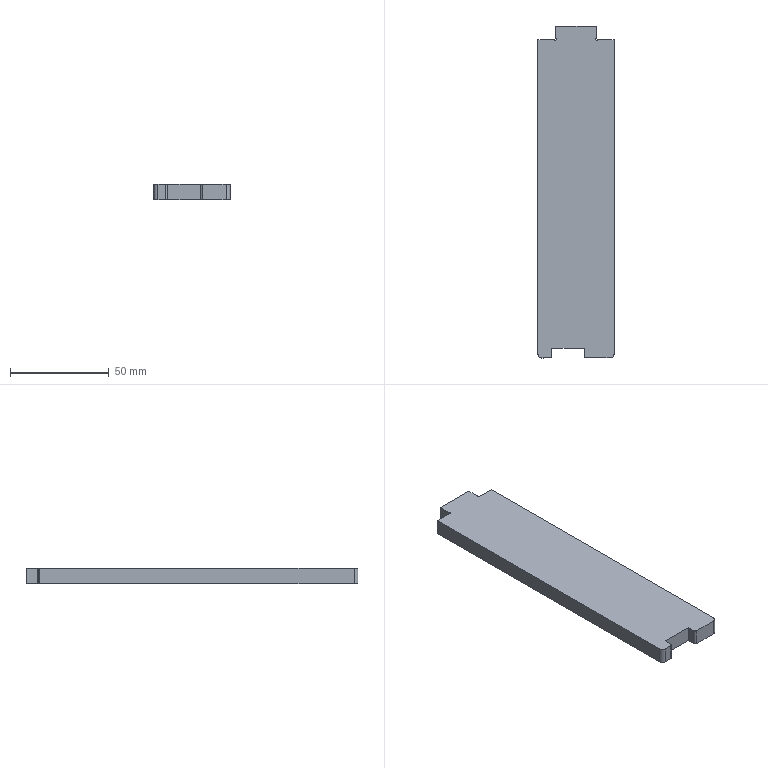Part | SolidWorks | features Fillet 2, FlatPattern 1, ICE 1, SMBaseFlange 1, SheetMetal 1 | 1 solid | 25 faces | box 38.5 x 167.8 x 8 mm | volume 49992 mm3 | plane 14 | cylinder 11 | commonest cylinder face diameters 2 x6 1 x3 4 x2
STEP:
#1=CARTESIAN_POINT('',(-109.914,161.326,-8.));
#2=VERTEX_POINT('',#1);
#3=CARTESIAN_POINT('',(-109.831,161.05,-8.));
#4=VERTEX_POINT('',#3);
#5=CARTESIAN_POINT('',(-110.331,161.05,-8.));
#6=DIRECTION('',(0.,0.,-1.));
#7=DIRECTION('',(-1.,0.,0.));
#8=AXIS2_PLACEMENT_3D('',#5,#6,#7);
#9=CIRCLE('',#8,0.5);
#10=EDGE_CURVE('',#2,#4,#9,.T.);
#11=ORIENTED_EDGE('',*,*,#10,.T.);
#12=CARTESIAN_POINT('',(-109.831,161.05,0.));
#13=VERTEX_POINT('',#12);
#14=CARTESIAN_POINT('',(-109.831,161.05,-8.));
#15=DIRECTION('',(0.,0.,1.));
#16=VECTOR('',#15,1000.);
#17=LINE('',#14,#16);
#18=EDGE_CURVE('',#4,#13,#17,.T.);
#19=ORIENTED_EDGE('',*,*,#18,.T.);
#20=CARTESIAN_POINT('',(-109.914,161.326,0.));
#21=VERTEX_POINT('',#20);
#22=CARTESIAN_POINT('',(-110.331,161.05,0.));
#23=DIRECTION('',(0.,0.,-1.));
#24=DIRECTION('',(-1.,0.,0.));
#25=AXIS2_PLACEMENT_3D('',#22,#23,#24);
#26=CIRCLE('',#25,0.5);
#27=EDGE_CURVE('',#21,#13,#26,.T.);
#28=ORIENTED_EDGE('',*,*,#27,.F.);
#29=CARTESIAN_POINT('',(-109.914,161.326,-8.));
#30=DIRECTION('',(0.,0.,-1.));
#31=VECTOR('',#30,1000.);
#32=LINE('',#29,#31);
#33=EDGE_CURVE('',#21,#2,#32,.T.);
#34=ORIENTED_EDGE('',*,*,#33,.T.);
#35=EDGE_LOOP('',(#11,#19,#28,#34));
#36=FACE_OUTER_BOUND('',#35,.T.);
#37=CARTESIAN_POINT('',(-110.331,161.05,-8.));
#38=DIRECTION('',(0.,0.,1.));
#39=DIRECTION('',(1.,0.,0.));
#40=AXIS2_PLACEMENT_3D('',#37,#38,#39);
#41=CYLINDRICAL_SURFACE('',#40,0.5);
#42=ADVANCED_FACE('',(#36),#41,.F.);
#43=CARTESIAN_POINT('',(-111.16,160.8,0.));
#44=VERTEX_POINT('',#43);
#45=CARTESIAN_POINT('',(-119.081,160.8,0.));
#46=VERTEX_POINT('',#45);
#47=CARTESIAN_POINT('',(-110.081,160.8,0.));
#48=DIRECTION('',(-1.,0.,0.));
#49=VECTOR('',#48,1000.);
#50=LINE('',#47,#49);
#51=EDGE_CURVE('',#44,#46,#50,.T.);
#52=ORIENTED_EDGE('',*,*,#51,.F.);
#53=CARTESIAN_POINT('',(-111.16,160.8,-8.));
#54=VERTEX_POINT('',#53);
#55=CARTESIAN_POINT('',(-111.16,160.8,-8.));
#56=DIRECTION('',(0.,0.,-1.));
#57=VECTOR('',#56,1000.);
#58=LINE('',#55,#57);
#59=EDGE_CURVE('',#44,#54,#58,.T.);
#60=ORIENTED_EDGE('',*,*,#59,.T.);
#61=CARTESIAN_POINT('',(-119.081,160.8,-8.));
#62=VERTEX_POINT('',#61);
#63=CARTESIAN_POINT('',(-110.081,160.8,-8.));
#64=DIRECTION('',(-1.,0.,0.));
#65=VECTOR('',#64,1000.);
#66=LINE('',#63,#65);
#67=EDGE_CURVE('',#54,#62,#66,.T.);
#68=ORIENTED_EDGE('',*,*,#67,.T.);
#69=CARTESIAN_POINT('',(-119.081,160.8,-8.));
#70=DIRECTION('',(0.,0.,1.));
#71=VECTOR('',#70,1000.);
#72=LINE('',#69,#71);
#73=EDGE_CURVE('',#62,#46,#72,.T.);
#74=ORIENTED_EDGE('',*,*,#73,.T.);
#75=EDGE_LOOP('',(#52,#60,#68,#74));
#76=FACE_OUTER_BOUND('',#75,.T.);
#77=CARTESIAN_POINT('',(-110.081,160.8,-8.));
#78=DIRECTION('',(0.,1.,0.));
#79=DIRECTION('',(0.,0.,1.));
#80=AXIS2_PLACEMENT_3D('',#77,#78,#79);
#81=PLANE('',#80);
#82=ADVANCED_FACE('',(#76),#81,.T.);
#83=CARTESIAN_POINT('',(-110.081,167.8,-8.));
#84=VERTEX_POINT('',#83);
#85=CARTESIAN_POINT('',(-110.081,161.879,-8.));
#86=VERTEX_POINT('',#85);
#87=CARTESIAN_POINT('',(-110.081,160.8,-8.));
#88=DIRECTION('',(0.,-1.,0.));
#89=VECTOR('',#88,1000.);
#90=LINE('',#87,#89);
#91=EDGE_CURVE('',#84,#86,#90,.T.);
#92=ORIENTED_EDGE('',*,*,#91,.T.);
#93=CARTESIAN_POINT('',(-110.081,161.879,0.));
#94=VERTEX_POINT('',#93);
#95=CARTESIAN_POINT('',(-110.081,161.879,-8.));
#96=DIRECTION('',(0.,0.,1.));
#97=VECTOR('',#96,1000.);
#98=LINE('',#95,#97);
#99=EDGE_CURVE('',#86,#94,#98,.T.);
#100=ORIENTED_EDGE('',*,*,#99,.T.);
#101=CARTESIAN_POINT('',(-110.081,167.8,0.));
#102=VERTEX_POINT('',#101);
#103=CARTESIAN_POINT('',(-110.081,160.8,0.));
#104=DIRECTION('',(0.,-1.,0.));
#105=VECTOR('',#104,1000.);
#106=LINE('',#103,#105);
#107=EDGE_CURVE('',#102,#94,#106,.T.);
#108=ORIENTED_EDGE('',*,*,#107,.F.);
#109=CARTESIAN_POINT('',(-110.081,167.8,-8.));
#110=DIRECTION('',(0.,0.,1.));
#111=VECTOR('',#110,1000.);
#112=LINE('',#109,#111);
#113=EDGE_CURVE('',#84,#102,#112,.T.);
#114=ORIENTED_EDGE('',*,*,#113,.F.);
#115=EDGE_LOOP('',(#92,#100,#108,#114));
#116=FACE_OUTER_BOUND('',#115,.T.);
#117=CARTESIAN_POINT('',(-110.081,160.8,-8.));
#118=DIRECTION('',(-1.,0.,0.));
#119=DIRECTION('',(0.,0.,1.));
#120=AXIS2_PLACEMENT_3D('',#117,#118,#119);
#121=PLANE('',#120);
#122=ADVANCED_FACE('',(#116),#121,.T.);
#123=CARTESIAN_POINT('',(-89.581,161.879,0.));
#124=VERTEX_POINT('',#123);
#125=CARTESIAN_POINT('',(-89.581,167.8,0.));
#126=VERTEX_POINT('',#125);
#127=CARTESIAN_POINT('',(-89.581,167.8,0.));
#128=DIRECTION('',(0.,1.,0.));
#129=VECTOR('',#128,1000.);
#130=LINE('',#127,#129);
#131=EDGE_CURVE('',#124,#126,#130,.T.);
#132=ORIENTED_EDGE('',*,*,#131,.F.);
#133=CARTESIAN_POINT('',(-89.581,161.879,-8.));
#134=VERTEX_POINT('',#133);
#135=CARTESIAN_POINT('',(-89.581,161.879,-8.));
#136=DIRECTION('',(0.,0.,-1.));
#137=VECTOR('',#136,1000.);
#138=LINE('',#135,#137);
#139=EDGE_CURVE('',#124,#134,#138,.T.);
#140=ORIENTED_EDGE('',*,*,#139,.T.);
#141=CARTESIAN_POINT('',(-89.581,167.8,-8.));
#142=VERTEX_POINT('',#141);
#143=CARTESIAN_POINT('',(-89.581,167.8,-8.));
#144=DIRECTION('',(0.,1.,0.));
#145=VECTOR('',#144,1000.);
#146=LINE('',#143,#145);
#147=EDGE_CURVE('',#134,#142,#146,.T.);
#148=ORIENTED_EDGE('',*,*,#147,.T.);
#149=CARTESIAN_POINT('',(-89.581,167.8,-8.));
#150=DIRECTION('',(0.,0.,1.));
#151=VECTOR('',#150,1000.);
#152=LINE('',#149,#151);
#153=EDGE_CURVE('',#142,#126,#152,.T.);
#154=ORIENTED_EDGE('',*,*,#153,.T.);
#155=EDGE_LOOP('',(#132,#140,#148,#154));
#156=FACE_OUTER_BOUND('',#155,.T.);
#157=CARTESIAN_POINT('',(-89.581,167.8,-8.));
#158=DIRECTION('',(1.,0.,0.));
#159=DIRECTION('',(0.,0.,-1.));
#160=AXIS2_PLACEMENT_3D('',#157,#158,#159);
#161=PLANE('',#160);
#162=ADVANCED_FACE('',(#156),#161,.T.);
#163=CARTESIAN_POINT('',(-80.581,160.8,-8.));
#164=VERTEX_POINT('',#163);
#165=CARTESIAN_POINT('',(-88.502,160.8,-8.));
#166=VERTEX_POINT('',#165);
#167=CARTESIAN_POINT('',(-80.581,160.8,-8.));
#168=DIRECTION('',(-1.,0.,0.));
#169=VECTOR('',#168,1000.);
#170=LINE('',#167,#169);
#171=EDGE_CURVE('',#164,#166,#170,.T.);
#172=ORIENTED_EDGE('',*,*,#171,.T.);
#173=CARTESIAN_POINT('',(-88.502,160.8,0.));
#174=VERTEX_POINT('',#173);
#175=CARTESIAN_POINT('',(-88.502,160.8,-8.));
#176=DIRECTION('',(0.,0.,1.));
#177=VECTOR('',#176,1000.);
#178=LINE('',#175,#177);
#179=EDGE_CURVE('',#166,#174,#178,.T.);
#180=ORIENTED_EDGE('',*,*,#179,.T.);
#181=CARTESIAN_POINT('',(-80.581,160.8,0.));
#182=VERTEX_POINT('',#181);
#183=CARTESIAN_POINT('',(-80.581,160.8,0.));
#184=DIRECTION('',(-1.,0.,0.));
#185=VECTOR('',#184,1000.);
#186=LINE('',#183,#185);
#187=EDGE_CURVE('',#182,#174,#186,.T.);
#188=ORIENTED_EDGE('',*,*,#187,.F.);
#189=CARTESIAN_POINT('',(-80.581,160.8,-8.));
#190=DIRECTION('',(0.,0.,1.));
#191=VECTOR('',#190,1000.);
#192=LINE('',#189,#191);
#193=EDGE_CURVE('',#164,#182,#192,.T.);
#194=ORIENTED_EDGE('',*,*,#193,.F.);
#195=EDGE_LOOP('',(#172,#180,#188,#194));
#196=FACE_OUTER_BOUND('',#195,.T.);
#197=CARTESIAN_POINT('',(-80.581,160.8,-8.));
#198=DIRECTION('',(0.,1.,0.));
#199=DIRECTION('',(0.,0.,1.));
#200=AXIS2_PLACEMENT_3D('',#197,#198,#199);
#201=PLANE('',#200);
#202=ADVANCED_FACE('',(#196),#201,.T.);
#203=CARTESIAN_POINT('',(-80.581,2.,-8.));
#204=VERTEX_POINT('',#203);
#205=CARTESIAN_POINT('',(-80.581,0.,-8.));
#206=DIRECTION('',(0.,1.,0.));
#207=VECTOR('',#206,1000.);
#208=LINE('',#205,#207);
#209=EDGE_CURVE('',#204,#164,#208,.T.);
#210=ORIENTED_EDGE('',*,*,#209,.F.);
#211=CARTESIAN_POINT('',(-82.581,0.,-8.));
#212=VERTEX_POINT('',#211);
#213=CARTESIAN_POINT('',(-82.581,2.,-8.));
#214=DIRECTION('',(0.,0.,-1.));
#215=DIRECTION('',(1.,0.,0.));
#216=AXIS2_PLACEMENT_3D('',#213,#214,#215);
#217=CIRCLE('',#216,2.);
#218=EDGE_CURVE('',#204,#212,#217,.T.);
#219=ORIENTED_EDGE('',*,*,#218,.T.);
#220=CARTESIAN_POINT('',(-94.581,0.,-8.));
#221=VERTEX_POINT('',#220);
#222=CARTESIAN_POINT('',(-95.581,0.,-8.));
#223=DIRECTION('',(1.,0.,0.));
#224=VECTOR('',#223,1000.);
#225=LINE('',#222,#224);
#226=EDGE_CURVE('',#221,#212,#225,.T.);
#227=ORIENTED_EDGE('',*,*,#226,.F.);
#228=CARTESIAN_POINT('',(-95.581,1.,-8.));
#229=VERTEX_POINT('',#228);
#230=CARTESIAN_POINT('',(-94.581,1.,-8.));
#231=DIRECTION('',(0.,0.,-1.));
#232=DIRECTION('',(1.,0.,0.));
#233=AXIS2_PLACEMENT_3D('',#230,#231,#232);
#234=CIRCLE('',#233,1.);
#235=EDGE_CURVE('',#221,#229,#234,.T.);
#236=ORIENTED_EDGE('',*,*,#235,.T.);
#237=CARTESIAN_POINT('',(-95.581,5.,-8.));
#238=VERTEX_POINT('',#237);
#239=CARTESIAN_POINT('',(-95.581,5.,-8.));
#240=DIRECTION('',(0.,-1.,0.));
#241=VECTOR('',#240,1000.);
#242=LINE('',#239,#241);
#243=EDGE_CURVE('',#238,#229,#242,.T.);
#244=ORIENTED_EDGE('',*,*,#243,.F.);
#245=CARTESIAN_POINT('',(-112.081,5.,-8.));
#246=VERTEX_POINT('',#245);
#247=CARTESIAN_POINT('',(-95.581,5.,-8.));
#248=DIRECTION('',(1.,0.,0.));
#249=VECTOR('',#248,1000.);
#250=LINE('',#247,#249);
#251=EDGE_CURVE('',#246,#238,#250,.T.);
#252=ORIENTED_EDGE('',*,*,#251,.F.);
#253=CARTESIAN_POINT('',(-112.081,1.,-8.));
#254=VERTEX_POINT('',#253);
#255=CARTESIAN_POINT('',(-112.081,5.,-8.));
#256=DIRECTION('',(0.,1.,0.));
#257=VECTOR('',#256,1000.);
#258=LINE('',#255,#257);
#259=EDGE_CURVE('',#254,#246,#258,.T.);
#260=ORIENTED_EDGE('',*,*,#259,.F.);
#261=CARTESIAN_POINT('',(-113.081,0.,-8.));
#262=VERTEX_POINT('',#261);
#263=CARTESIAN_POINT('',(-113.081,1.,-8.));
#264=DIRECTION('',(0.,0.,-1.));
#265=DIRECTION('',(1.,0.,0.));
#266=AXIS2_PLACEMENT_3D('',#263,#264,#265);
#267=CIRCLE('',#266,1.);
#268=EDGE_CURVE('',#254,#262,#267,.T.);
#269=ORIENTED_EDGE('',*,*,#268,.T.);
#270=CARTESIAN_POINT('',(-117.081,0.,-8.));
#271=VERTEX_POINT('',#270);
#272=CARTESIAN_POINT('',(-112.081,0.,-8.));
#273=DIRECTION('',(1.,0.,0.));
#274=VECTOR('',#273,1000.);
#275=LINE('',#272,#274);
#276=EDGE_CURVE('',#271,#262,#275,.T.);
#277=ORIENTED_EDGE('',*,*,#276,.F.);
#278=CARTESIAN_POINT('',(-119.081,2.,-8.));
#279=VERTEX_POINT('',#278);
#280=CARTESIAN_POINT('',(-117.081,2.,-8.));
#281=DIRECTION('',(0.,0.,-1.));
#282=DIRECTION('',(1.,0.,0.));
#283=AXIS2_PLACEMENT_3D('',#280,#281,#282);
#284=CIRCLE('',#283,2.);
#285=EDGE_CURVE('',#271,#279,#284,.T.);
#286=ORIENTED_EDGE('',*,*,#285,.T.);
#287=CARTESIAN_POINT('',(-119.081,0.,-8.));
#288=DIRECTION('',(0.,-1.,0.));
#289=VECTOR('',#288,1000.);
#290=LINE('',#287,#289);
#291=EDGE_CURVE('',#62,#279,#290,.T.);
#292=ORIENTED_EDGE('',*,*,#291,.F.);
#293=ORIENTED_EDGE('',*,*,#67,.F.);
#294=CARTESIAN_POINT('',(-110.607,160.633,-8.));
#295=VERTEX_POINT('',#294);
#296=CARTESIAN_POINT('',(-111.16,159.8,-8.));
#297=DIRECTION('',(0.,0.,-1.));
#298=DIRECTION('',(1.,0.,0.));
#299=AXIS2_PLACEMENT_3D('',#296,#297,#298);
#300=CIRCLE('',#299,1.);
#301=EDGE_CURVE('',#54,#295,#300,.T.);
#302=ORIENTED_EDGE('',*,*,#301,.T.);
#303=CARTESIAN_POINT('',(-110.331,161.05,-8.));
#304=DIRECTION('',(0.,0.,-1.));
#305=DIRECTION('',(-1.,0.,0.));
#306=AXIS2_PLACEMENT_3D('',#303,#304,#305);
#307=CIRCLE('',#306,0.5);
#308=EDGE_CURVE('',#4,#295,#307,.T.);
#309=ORIENTED_EDGE('',*,*,#308,.F.);
#310=ORIENTED_EDGE('',*,*,#10,.F.);
#311=CARTESIAN_POINT('',(-109.081,161.879,-8.));
#312=DIRECTION('',(0.,0.,-1.));
#313=DIRECTION('',(1.,0.,0.));
#314=AXIS2_PLACEMENT_3D('',#311,#312,#313);
#315=CIRCLE('',#314,1.);
#316=EDGE_CURVE('',#2,#86,#315,.T.);
#317=ORIENTED_EDGE('',*,*,#316,.T.);
#318=ORIENTED_EDGE('',*,*,#91,.F.);
#319=CARTESIAN_POINT('',(-110.081,167.8,-8.));
#320=DIRECTION('',(-1.,0.,0.));
#321=VECTOR('',#320,1000.);
#322=LINE('',#319,#321);
#323=EDGE_CURVE('',#142,#84,#322,.T.);
#324=ORIENTED_EDGE('',*,*,#323,.F.);
#325=ORIENTED_EDGE('',*,*,#147,.F.);
#326=CARTESIAN_POINT('',(-89.747,161.326,-8.));
#327=VERTEX_POINT('',#326);
#328=CARTESIAN_POINT('',(-90.581,161.879,-8.));
#329=DIRECTION('',(0.,0.,-1.));
#330=DIRECTION('',(1.,0.,0.));
#331=AXIS2_PLACEMENT_3D('',#328,#329,#330);
#332=CIRCLE('',#331,1.);
#333=EDGE_CURVE('',#134,#327,#332,.T.);
#334=ORIENTED_EDGE('',*,*,#333,.T.);
#335=CARTESIAN_POINT('',(-89.054,160.633,-8.));
#336=VERTEX_POINT('',#335);
#337=CARTESIAN_POINT('',(-89.331,161.05,-8.));
#338=DIRECTION('',(0.,0.,-1.));
#339=DIRECTION('',(-1.,0.,0.));
#340=AXIS2_PLACEMENT_3D('',#337,#338,#339);
#341=CIRCLE('',#340,0.5);
#342=EDGE_CURVE('',#336,#327,#341,.T.);
#343=ORIENTED_EDGE('',*,*,#342,.F.);
#344=CARTESIAN_POINT('',(-88.502,159.8,-8.));
#345=DIRECTION('',(0.,0.,-1.));
#346=DIRECTION('',(1.,0.,0.));
#347=AXIS2_PLACEMENT_3D('',#344,#345,#346);
#348=CIRCLE('',#347,1.);
#349=EDGE_CURVE('',#336,#166,#348,.T.);
#350=ORIENTED_EDGE('',*,*,#349,.T.);
#351=ORIENTED_EDGE('',*,*,#171,.F.);
#352=EDGE_LOOP('',(#210,#219,#227,#236,#244,#252,#260,#269,#277,#286,#292,#293,#302,#309,#310,#317,#318,#324,#325,#334,#343,#350,#351));
#353=FACE_OUTER_BOUND('',#352,.T.);
#354=CARTESIAN_POINT('',(0.,0.,-8.));
#355=DIRECTION('',(0.,0.,1.));
#356=DIRECTION('',(1.,0.,0.));
#357=AXIS2_PLACEMENT_3D('',#354,#355,#356);
#358=PLANE('',#357);
#359=ADVANCED_FACE('',(#353),#358,.F.);
#360=CARTESIAN_POINT('',(-94.581,0.,0.));
#361=VERTEX_POINT('',#360);
#362=CARTESIAN_POINT('',(-82.581,0.,0.));
#363=VERTEX_POINT('',#362);
#364=CARTESIAN_POINT('',(-95.581,0.,0.));
#365=DIRECTION('',(1.,0.,0.));
#366=VECTOR('',#365,1000.);
#367=LINE('',#364,#366);
#368=EDGE_CURVE('',#361,#363,#367,.T.);
#369=ORIENTED_EDGE('',*,*,#368,.T.);
#370=CARTESIAN_POINT('',(-80.581,2.,0.));
#371=VERTEX_POINT('',#370);
#372=CARTESIAN_POINT('',(-82.581,2.,0.));
#373=DIRECTION('',(0.,0.,1.));
#374=DIRECTION('',(1.,0.,0.));
#375=AXIS2_PLACEMENT_3D('',#372,#373,#374);
#376=CIRCLE('',#375,2.);
#377=EDGE_CURVE('',#363,#371,#376,.T.);
#378=ORIENTED_EDGE('',*,*,#377,.T.);
#379=CARTESIAN_POINT('',(-80.581,0.,0.));
#380=DIRECTION('',(0.,1.,0.));
#381=VECTOR('',#380,1000.);
#382=LINE('',#379,#381);
#383=EDGE_CURVE('',#371,#182,#382,.T.);
#384=ORIENTED_EDGE('',*,*,#383,.T.);
#385=ORIENTED_EDGE('',*,*,#187,.T.);
#386=CARTESIAN_POINT('',(-89.054,160.633,0.));
#387=VERTEX_POINT('',#386);
#388=CARTESIAN_POINT('',(-88.502,159.8,0.));
#389=DIRECTION('',(0.,0.,1.));
#390=DIRECTION('',(1.,0.,0.));
#391=AXIS2_PLACEMENT_3D('',#388,#389,#390);
#392=CIRCLE('',#391,1.);
#393=EDGE_CURVE('',#174,#387,#392,.T.);
#394=ORIENTED_EDGE('',*,*,#393,.T.);
#395=CARTESIAN_POINT('',(-89.747,161.326,0.));
#396=VERTEX_POINT('',#395);
#397=CARTESIAN_POINT('',(-89.331,161.05,0.));
#398=DIRECTION('',(0.,0.,-1.));
#399=DIRECTION('',(-1.,0.,0.));
#400=AXIS2_PLACEMENT_3D('',#397,#398,#399);
#401=CIRCLE('',#400,0.5);
#402=EDGE_CURVE('',#387,#396,#401,.T.);
#403=ORIENTED_EDGE('',*,*,#402,.T.);
#404=CARTESIAN_POINT('',(-90.581,161.879,0.));
#405=DIRECTION('',(0.,0.,1.));
#406=DIRECTION('',(1.,0.,0.));
#407=AXIS2_PLACEMENT_3D('',#404,#405,#406);
#408=CIRCLE('',#407,1.);
#409=EDGE_CURVE('',#396,#124,#408,.T.);
#410=ORIENTED_EDGE('',*,*,#409,.T.);
#411=ORIENTED_EDGE('',*,*,#131,.T.);
#412=CARTESIAN_POINT('',(-110.081,167.8,0.));
#413=DIRECTION('',(-1.,0.,0.));
#414=VECTOR('',#413,1000.);
#415=LINE('',#412,#414);
#416=EDGE_CURVE('',#126,#102,#415,.T.);
#417=ORIENTED_EDGE('',*,*,#416,.T.);
#418=ORIENTED_EDGE('',*,*,#107,.T.);
#419=CARTESIAN_POINT('',(-109.081,161.879,0.));
#420=DIRECTION('',(0.,0.,1.));
#421=DIRECTION('',(1.,0.,0.));
#422=AXIS2_PLACEMENT_3D('',#419,#420,#421);
#423=CIRCLE('',#422,1.);
#424=EDGE_CURVE('',#94,#21,#423,.T.);
#425=ORIENTED_EDGE('',*,*,#424,.T.);
#426=ORIENTED_EDGE('',*,*,#27,.T.);
#427=CARTESIAN_POINT('',(-110.607,160.633,0.));
#428=VERTEX_POINT('',#427);
#429=CARTESIAN_POINT('',(-110.331,161.05,0.));
#430=DIRECTION('',(0.,0.,-1.));
#431=DIRECTION('',(-1.,0.,0.));
#432=AXIS2_PLACEMENT_3D('',#429,#430,#431);
#433=CIRCLE('',#432,0.5);
#434=EDGE_CURVE('',#13,#428,#433,.T.);
#435=ORIENTED_EDGE('',*,*,#434,.T.);
#436=CARTESIAN_POINT('',(-111.16,159.8,0.));
#437=DIRECTION('',(0.,0.,1.));
#438=DIRECTION('',(1.,0.,0.));
#439=AXIS2_PLACEMENT_3D('',#436,#437,#438);
#440=CIRCLE('',#439,1.);
#441=EDGE_CURVE('',#428,#44,#440,.T.);
#442=ORIENTED_EDGE('',*,*,#441,.T.);
#443=ORIENTED_EDGE('',*,*,#51,.T.);
#444=CARTESIAN_POINT('',(-119.081,2.,0.));
#445=VERTEX_POINT('',#444);
#446=CARTESIAN_POINT('',(-119.081,0.,0.));
#447=DIRECTION('',(0.,-1.,0.));
#448=VECTOR('',#447,1000.);
#449=LINE('',#446,#448);
#450=EDGE_CURVE('',#46,#445,#449,.T.);
#451=ORIENTED_EDGE('',*,*,#450,.T.);
#452=CARTESIAN_POINT('',(-117.081,0.,0.));
#453=VERTEX_POINT('',#452);
#454=CARTESIAN_POINT('',(-117.081,2.,0.));
#455=DIRECTION('',(0.,0.,1.));
#456=DIRECTION('',(1.,0.,0.));
#457=AXIS2_PLACEMENT_3D('',#454,#455,#456);
#458=CIRCLE('',#457,2.);
#459=EDGE_CURVE('',#445,#453,#458,.T.);
#460=ORIENTED_EDGE('',*,*,#459,.T.);
#461=CARTESIAN_POINT('',(-113.081,0.,0.));
#462=VERTEX_POINT('',#461);
#463=CARTESIAN_POINT('',(-112.081,0.,0.));
#464=DIRECTION('',(1.,0.,0.));
#465=VECTOR('',#464,1000.);
#466=LINE('',#463,#465);
#467=EDGE_CURVE('',#453,#462,#466,.T.);
#468=ORIENTED_EDGE('',*,*,#467,.T.);
#469=CARTESIAN_POINT('',(-112.081,1.,0.));
#470=VERTEX_POINT('',#469);
#471=CARTESIAN_POINT('',(-113.081,1.,0.));
#472=DIRECTION('',(0.,0.,1.));
#473=DIRECTION('',(1.,0.,0.));
#474=AXIS2_PLACEMENT_3D('',#471,#472,#473);
#475=CIRCLE('',#474,1.);
#476=EDGE_CURVE('',#462,#470,#475,.T.);
#477=ORIENTED_EDGE('',*,*,#476,.T.);
#478=CARTESIAN_POINT('',(-112.081,5.,0.));
#479=VERTEX_POINT('',#478);
#480=CARTESIAN_POINT('',(-112.081,5.,0.));
#481=DIRECTION('',(0.,1.,0.));
#482=VECTOR('',#481,1000.);
#483=LINE('',#480,#482);
#484=EDGE_CURVE('',#470,#479,#483,.T.);
#485=ORIENTED_EDGE('',*,*,#484,.T.);
#486=CARTESIAN_POINT('',(-95.581,5.,0.));
#487=VERTEX_POINT('',#486);
#488=CARTESIAN_POINT('',(-95.581,5.,0.));
#489=DIRECTION('',(1.,0.,0.));
#490=VECTOR('',#489,1000.);
#491=LINE('',#488,#490);
#492=EDGE_CURVE('',#479,#487,#491,.T.);
#493=ORIENTED_EDGE('',*,*,#492,.T.);
#494=CARTESIAN_POINT('',(-95.581,1.,0.));
#495=VERTEX_POINT('',#494);
#496=CARTESIAN_POINT('',(-95.581,5.,0.));
#497=DIRECTION('',(0.,-1.,0.));
#498=VECTOR('',#497,1000.);
#499=LINE('',#496,#498);
#500=EDGE_CURVE('',#487,#495,#499,.T.);
#501=ORIENTED_EDGE('',*,*,#500,.T.);
#502=CARTESIAN_POINT('',(-94.581,1.,0.));
#503=DIRECTION('',(0.,0.,1.));
#504=DIRECTION('',(1.,0.,0.));
#505=AXIS2_PLACEMENT_3D('',#502,#503,#504);
#506=CIRCLE('',#505,1.);
#507=EDGE_CURVE('',#495,#361,#506,.T.);
#508=ORIENTED_EDGE('',*,*,#507,.T.);
#509=EDGE_LOOP('',(#369,#378,#384,#385,#394,#403,#410,#411,#417,#418,#425,#426,#435,#442,#443,#451,#460,#468,#477,#485,#493,#501,#508));
#510=FACE_OUTER_BOUND('',#509,.T.);
#511=CARTESIAN_POINT('',(0.,0.,0.));
#512=DIRECTION('',(0.,0.,1.));
#513=DIRECTION('',(1.,0.,0.));
#514=AXIS2_PLACEMENT_3D('',#511,#512,#513);
#515=PLANE('',#514);
#516=ADVANCED_FACE('',(#510),#515,.T.);
#517=ORIENTED_EDGE('',*,*,#383,.F.);
#518=CARTESIAN_POINT('',(-80.581,2.,-8.));
#519=DIRECTION('',(0.,0.,-1.));
#520=VECTOR('',#519,1000.);
#521=LINE('',#518,#520);
#522=EDGE_CURVE('',#371,#204,#521,.T.);
#523=ORIENTED_EDGE('',*,*,#522,.T.);
#524=ORIENTED_EDGE('',*,*,#209,.T.);
#525=ORIENTED_EDGE('',*,*,#193,.T.);
#526=EDGE_LOOP('',(#517,#523,#524,#525));
#527=FACE_OUTER_BOUND('',#526,.T.);
#528=CARTESIAN_POINT('',(-80.581,0.,-8.));
#529=DIRECTION('',(1.,0.,0.));
#530=DIRECTION('',(0.,1.,0.));
#531=AXIS2_PLACEMENT_3D('',#528,#529,#530);
#532=PLANE('',#531);
#533=ADVANCED_FACE('',(#527),#532,.T.);
#534=ORIENTED_EDGE('',*,*,#226,.T.);
#535=CARTESIAN_POINT('',(-82.581,0.,-8.));
#536=DIRECTION('',(0.,0.,1.));
#537=VECTOR('',#536,1000.);
#538=LINE('',#535,#537);
#539=EDGE_CURVE('',#212,#363,#538,.T.);
#540=ORIENTED_EDGE('',*,*,#539,.T.);
#541=ORIENTED_EDGE('',*,*,#368,.F.);
#542=CARTESIAN_POINT('',(-94.581,0.,-8.));
#543=DIRECTION('',(0.,0.,-1.));
#544=VECTOR('',#543,1000.);
#545=LINE('',#542,#544);
#546=EDGE_CURVE('',#361,#221,#545,.T.);
#547=ORIENTED_EDGE('',*,*,#546,.T.);
#548=EDGE_LOOP('',(#534,#540,#541,#547));
#549=FACE_OUTER_BOUND('',#548,.T.);
#550=CARTESIAN_POINT('',(-95.581,0.,-8.));
#551=DIRECTION('',(0.,-1.,0.));
#552=DIRECTION('',(1.,0.,0.));
#553=AXIS2_PLACEMENT_3D('',#550,#551,#552);
#554=PLANE('',#553);
#555=ADVANCED_FACE('',(#549),#554,.T.);
#556=ORIENTED_EDGE('',*,*,#243,.T.);
#557=CARTESIAN_POINT('',(-95.581,1.,-8.));
#558=DIRECTION('',(0.,0.,1.));
#559=VECTOR('',#558,1000.);
#560=LINE('',#557,#559);
#561=EDGE_CURVE('',#229,#495,#560,.T.);
#562=ORIENTED_EDGE('',*,*,#561,.T.);
#563=ORIENTED_EDGE('',*,*,#500,.F.);
#564=CARTESIAN_POINT('',(-95.581,5.,-8.));
#565=DIRECTION('',(0.,0.,1.));
#566=VECTOR('',#565,1000.);
#567=LINE('',#564,#566);
#568=EDGE_CURVE('',#238,#487,#567,.T.);
#569=ORIENTED_EDGE('',*,*,#568,.F.);
#570=EDGE_LOOP('',(#556,#562,#563,#569));
#571=FACE_OUTER_BOUND('',#570,.T.);
#572=CARTESIAN_POINT('',(-95.581,5.,-8.));
#573=DIRECTION('',(-1.,0.,0.));
#574=DIRECTION('',(0.,0.,1.));
#575=AXIS2_PLACEMENT_3D('',#572,#573,#574);
#576=PLANE('',#575);
#577=ADVANCED_FACE('',(#571),#576,.T.);
#578=ORIENTED_EDGE('',*,*,#492,.F.);
#579=CARTESIAN_POINT('',(-112.081,5.,-8.));
#580=DIRECTION('',(0.,0.,1.));
#581=VECTOR('',#580,1000.);
#582=LINE('',#579,#581);
#583=EDGE_CURVE('',#246,#479,#582,.T.);
#584=ORIENTED_EDGE('',*,*,#583,.F.);
#585=ORIENTED_EDGE('',*,*,#251,.T.);
#586=ORIENTED_EDGE('',*,*,#568,.T.);
#587=EDGE_LOOP('',(#578,#584,#585,#586));
#588=FACE_OUTER_BOUND('',#587,.T.);
#589=CARTESIAN_POINT('',(-95.581,5.,-8.));
#590=DIRECTION('',(0.,-1.,0.));
#591=DIRECTION('',(1.,0.,0.));
#592=AXIS2_PLACEMENT_3D('',#589,#590,#591);
#593=PLANE('',#592);
#594=ADVANCED_FACE('',(#588),#593,.T.);
#595=ORIENTED_EDGE('',*,*,#484,.F.);
#596=CARTESIAN_POINT('',(-112.081,1.,-8.));
#597=DIRECTION('',(0.,0.,-1.));
#598=VECTOR('',#597,1000.);
#599=LINE('',#596,#598);
#600=EDGE_CURVE('',#470,#254,#599,.T.);
#601=ORIENTED_EDGE('',*,*,#600,.T.);
#602=ORIENTED_EDGE('',*,*,#259,.T.);
#603=ORIENTED_EDGE('',*,*,#583,.T.);
#604=EDGE_LOOP('',(#595,#601,#602,#603));
#605=FACE_OUTER_BOUND('',#604,.T.);
#606=CARTESIAN_POINT('',(-112.081,5.,-8.));
#607=DIRECTION('',(1.,0.,0.));
#608=DIRECTION('',(0.,0.,-1.));
#609=AXIS2_PLACEMENT_3D('',#606,#607,#608);
#610=PLANE('',#609);
#611=ADVANCED_FACE('',(#605),#610,.T.);
#612=ORIENTED_EDGE('',*,*,#467,.F.);
#613=CARTESIAN_POINT('',(-117.081,0.,-8.));
#614=DIRECTION('',(0.,0.,-1.));
#615=VECTOR('',#614,1000.);
#616=LINE('',#613,#615);
#617=EDGE_CURVE('',#453,#271,#616,.T.);
#618=ORIENTED_EDGE('',*,*,#617,.T.);
#619=ORIENTED_EDGE('',*,*,#276,.T.);
#620=CARTESIAN_POINT('',(-113.081,0.,-8.));
#621=DIRECTION('',(0.,0.,1.));
#622=VECTOR('',#621,1000.);
#623=LINE('',#620,#622);
#624=EDGE_CURVE('',#262,#462,#623,.T.);
#625=ORIENTED_EDGE('',*,*,#624,.T.);
#626=EDGE_LOOP('',(#612,#618,#619,#625));
#627=FACE_OUTER_BOUND('',#626,.T.);
#628=CARTESIAN_POINT('',(-112.081,0.,-8.));
#629=DIRECTION('',(0.,-1.,0.));
#630=DIRECTION('',(1.,0.,0.));
#631=AXIS2_PLACEMENT_3D('',#628,#629,#630);
#632=PLANE('',#631);
#633=ADVANCED_FACE('',(#627),#632,.T.);
#634=ORIENTED_EDGE('',*,*,#291,.T.);
#635=CARTESIAN_POINT('',(-119.081,2.,-8.));
#636=DIRECTION('',(0.,0.,1.));
#637=VECTOR('',#636,1000.);
#638=LINE('',#635,#637);
#639=EDGE_CURVE('',#279,#445,#638,.T.);
#640=ORIENTED_EDGE('',*,*,#639,.T.);
#641=ORIENTED_EDGE('',*,*,#450,.F.);
#642=ORIENTED_EDGE('',*,*,#73,.F.);
#643=EDGE_LOOP('',(#634,#640,#641,#642));
#644=FACE_OUTER_BOUND('',#643,.T.);
#645=CARTESIAN_POINT('',(-119.081,0.,-8.));
#646=DIRECTION('',(-1.,0.,0.));
#647=DIRECTION('',(0.,-1.,0.));
#648=AXIS2_PLACEMENT_3D('',#645,#646,#647);
#649=PLANE('',#648);
#650=ADVANCED_FACE('',(#644),#649,.T.);
#651=ORIENTED_EDGE('',*,*,#416,.F.);
#652=ORIENTED_EDGE('',*,*,#153,.F.);
#653=ORIENTED_EDGE('',*,*,#323,.T.);
#654=ORIENTED_EDGE('',*,*,#113,.T.);
#655=EDGE_LOOP('',(#651,#652,#653,#654));
#656=FACE_OUTER_BOUND('',#655,.T.);
#657=CARTESIAN_POINT('',(-110.081,167.8,-8.));
#658=DIRECTION('',(0.,1.,0.));
#659=DIRECTION('',(0.,0.,1.));
#660=AXIS2_PLACEMENT_3D('',#657,#658,#659);
#661=PLANE('',#660);
#662=ADVANCED_FACE('',(#656),#661,.T.);
#663=ORIENTED_EDGE('',*,*,#402,.F.);
#664=CARTESIAN_POINT('',(-89.054,160.633,-8.));
#665=DIRECTION('',(0.,0.,-1.));
#666=VECTOR('',#665,1000.);
#667=LINE('',#664,#666);
#668=EDGE_CURVE('',#387,#336,#667,.T.);
#669=ORIENTED_EDGE('',*,*,#668,.T.);
#670=ORIENTED_EDGE('',*,*,#342,.T.);
#671=CARTESIAN_POINT('',(-89.747,161.326,-8.));
#672=DIRECTION('',(0.,0.,1.));
#673=VECTOR('',#672,1000.);
#674=LINE('',#671,#673);
#675=EDGE_CURVE('',#327,#396,#674,.T.);
#676=ORIENTED_EDGE('',*,*,#675,.T.);
#677=EDGE_LOOP('',(#663,#669,#670,#676));
#678=FACE_OUTER_BOUND('',#677,.T.);
#679=CARTESIAN_POINT('',(-89.331,161.05,-8.));
#680=DIRECTION('',(0.,0.,1.));
#681=DIRECTION('',(1.,0.,0.));
#682=AXIS2_PLACEMENT_3D('',#679,#680,#681);
#683=CYLINDRICAL_SURFACE('',#682,0.5);
#684=ADVANCED_FACE('',(#678),#683,.F.);
#685=ORIENTED_EDGE('',*,*,#18,.F.);
#686=ORIENTED_EDGE('',*,*,#308,.T.);
#687=CARTESIAN_POINT('',(-110.607,160.633,-8.));
#688=DIRECTION('',(0.,0.,1.));
#689=VECTOR('',#688,1000.);
#690=LINE('',#687,#689);
#691=EDGE_CURVE('',#295,#428,#690,.T.);
#692=ORIENTED_EDGE('',*,*,#691,.T.);
#693=ORIENTED_EDGE('',*,*,#434,.F.);
#694=EDGE_LOOP('',(#685,#686,#692,#693));
#695=FACE_OUTER_BOUND('',#694,.T.);
#696=CARTESIAN_POINT('',(-110.331,161.05,-8.));
#697=DIRECTION('',(0.,0.,1.));
#698=DIRECTION('',(1.,0.,0.));
#699=AXIS2_PLACEMENT_3D('',#696,#697,#698);
#700=CYLINDRICAL_SURFACE('',#699,0.5);
#701=ADVANCED_FACE('',(#695),#700,.F.);
#702=ORIENTED_EDGE('',*,*,#268,.F.);
#703=ORIENTED_EDGE('',*,*,#600,.F.);
#704=ORIENTED_EDGE('',*,*,#476,.F.);
#705=ORIENTED_EDGE('',*,*,#624,.F.);
#706=EDGE_LOOP('',(#702,#703,#704,#705));
#707=FACE_OUTER_BOUND('',#706,.T.);
#708=CARTESIAN_POINT('',(-113.081,1.,-8.));
#709=DIRECTION('',(0.,0.,1.));
#710=DIRECTION('',(1.,0.,0.));
#711=AXIS2_PLACEMENT_3D('',#708,#709,#710);
#712=CYLINDRICAL_SURFACE('',#711,1.);
#713=ADVANCED_FACE('',(#707),#712,.T.);
#714=ORIENTED_EDGE('',*,*,#235,.F.);
#715=ORIENTED_EDGE('',*,*,#546,.F.);
#716=ORIENTED_EDGE('',*,*,#507,.F.);
#717=ORIENTED_EDGE('',*,*,#561,.F.);
#718=EDGE_LOOP('',(#714,#715,#716,#717));
#719=FACE_OUTER_BOUND('',#718,.T.);
#720=CARTESIAN_POINT('',(-94.581,1.,-8.));
#721=DIRECTION('',(0.,0.,1.));
#722=DIRECTION('',(1.,0.,0.));
#723=AXIS2_PLACEMENT_3D('',#720,#721,#722);
#724=CYLINDRICAL_SURFACE('',#723,1.);
#725=ADVANCED_FACE('',(#719),#724,.T.);
#726=ORIENTED_EDGE('',*,*,#349,.F.);
#727=ORIENTED_EDGE('',*,*,#668,.F.);
#728=ORIENTED_EDGE('',*,*,#393,.F.);
#729=ORIENTED_EDGE('',*,*,#179,.F.);
#730=EDGE_LOOP('',(#726,#727,#728,#729));
#731=FACE_OUTER_BOUND('',#730,.T.);
#732=CARTESIAN_POINT('',(-88.502,159.8,-8.));
#733=DIRECTION('',(0.,0.,1.));
#734=DIRECTION('',(1.,0.,0.));
#735=AXIS2_PLACEMENT_3D('',#732,#733,#734);
#736=CYLINDRICAL_SURFACE('',#735,1.);
#737=ADVANCED_FACE('',(#731),#736,.T.);
#738=ORIENTED_EDGE('',*,*,#333,.F.);
#739=ORIENTED_EDGE('',*,*,#139,.F.);
#740=ORIENTED_EDGE('',*,*,#409,.F.);
#741=ORIENTED_EDGE('',*,*,#675,.F.);
#742=EDGE_LOOP('',(#738,#739,#740,#741));
#743=FACE_OUTER_BOUND('',#742,.T.);
#744=CARTESIAN_POINT('',(-90.581,161.879,-8.));
#745=DIRECTION('',(0.,0.,1.));
#746=DIRECTION('',(1.,0.,0.));
#747=AXIS2_PLACEMENT_3D('',#744,#745,#746);
#748=CYLINDRICAL_SURFACE('',#747,1.);
#749=ADVANCED_FACE('',(#743),#748,.T.);
#750=ORIENTED_EDGE('',*,*,#316,.F.);
#751=ORIENTED_EDGE('',*,*,#33,.F.);
#752=ORIENTED_EDGE('',*,*,#424,.F.);
#753=ORIENTED_EDGE('',*,*,#99,.F.);
#754=EDGE_LOOP('',(#750,#751,#752,#753));
#755=FACE_OUTER_BOUND('',#754,.T.);
#756=CARTESIAN_POINT('',(-109.081,161.879,-8.));
#757=DIRECTION('',(0.,0.,1.));
#758=DIRECTION('',(1.,0.,0.));
#759=AXIS2_PLACEMENT_3D('',#756,#757,#758);
#760=CYLINDRICAL_SURFACE('',#759,1.);
#761=ADVANCED_FACE('',(#755),#760,.T.);
#762=ORIENTED_EDGE('',*,*,#301,.F.);
#763=ORIENTED_EDGE('',*,*,#59,.F.);
#764=ORIENTED_EDGE('',*,*,#441,.F.);
#765=ORIENTED_EDGE('',*,*,#691,.F.);
#766=EDGE_LOOP('',(#762,#763,#764,#765));
#767=FACE_OUTER_BOUND('',#766,.T.);
#768=CARTESIAN_POINT('',(-111.16,159.8,-8.));
#769=DIRECTION('',(0.,0.,1.));
#770=DIRECTION('',(1.,0.,0.));
#771=AXIS2_PLACEMENT_3D('',#768,#769,#770);
#772=CYLINDRICAL_SURFACE('',#771,1.);
#773=ADVANCED_FACE('',(#767),#772,.T.);
#774=ORIENTED_EDGE('',*,*,#218,.F.);
#775=ORIENTED_EDGE('',*,*,#522,.F.);
#776=ORIENTED_EDGE('',*,*,#377,.F.);
#777=ORIENTED_EDGE('',*,*,#539,.F.);
#778=EDGE_LOOP('',(#774,#775,#776,#777));
#779=FACE_OUTER_BOUND('',#778,.T.);
#780=CARTESIAN_POINT('',(-82.581,2.,-8.));
#781=DIRECTION('',(0.,0.,1.));
#782=DIRECTION('',(1.,0.,0.));
#783=AXIS2_PLACEMENT_3D('',#780,#781,#782);
#784=CYLINDRICAL_SURFACE('',#783,2.);
#785=ADVANCED_FACE('',(#779),#784,.T.);
#786=ORIENTED_EDGE('',*,*,#285,.F.);
#787=ORIENTED_EDGE('',*,*,#617,.F.);
#788=ORIENTED_EDGE('',*,*,#459,.F.);
#789=ORIENTED_EDGE('',*,*,#639,.F.);
#790=EDGE_LOOP('',(#786,#787,#788,#789));
#791=FACE_OUTER_BOUND('',#790,.T.);
#792=CARTESIAN_POINT('',(-117.081,2.,-8.));
#793=DIRECTION('',(0.,0.,1.));
#794=DIRECTION('',(1.,0.,0.));
#795=AXIS2_PLACEMENT_3D('',#792,#793,#794);
#796=CYLINDRICAL_SURFACE('',#795,2.);
#797=ADVANCED_FACE('',(#791),#796,.T.);
#798=CLOSED_SHELL('',(#42,#82,#122,#162,#202,#359,#516,#533,#555,#577,#594,#611,#633,#650,#662,#684,#701,#713,#725,#737,#749,#761,#773,#785,#797));
#799=MANIFOLD_SOLID_BREP('',#798);
#800=CARTESIAN_POINT('',(0.,0.,0.));
#801=DIRECTION('',(0.,0.,1.));
#802=DIRECTION('',(1.,0.,0.));
#803=AXIS2_PLACEMENT_3D('',#800,#801,#802);
#804=(LENGTH_UNIT()NAMED_UNIT(*)SI_UNIT(.MILLI.,.METRE.));
#805=UNCERTAINTY_MEASURE_WITH_UNIT(LENGTH_MEASURE(0.00001),#804,'','');
#806=(NAMED_UNIT(*)PLANE_ANGLE_UNIT()SI_UNIT($,.RADIAN.));
#807=(NAMED_UNIT(*)SI_UNIT($,.STERADIAN.)SOLID_ANGLE_UNIT());
#808=(GEOMETRIC_REPRESENTATION_CONTEXT(3)GLOBAL_UNCERTAINTY_ASSIGNED_CONTEXT((#805))GLOBAL_UNIT_ASSIGNED_CONTEXT((#804,#806,#807))REPRESENTATION_CONTEXT('',''));
#809=ADVANCED_BREP_SHAPE_REPRESENTATION('',(#799,#803),#808);